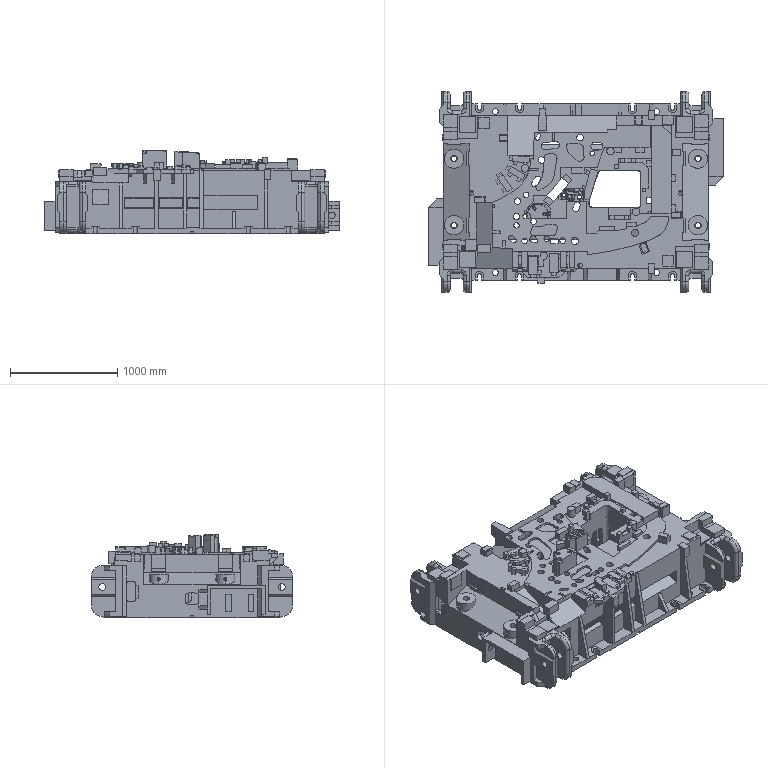Part | NX | features solid 2 | 1 solid | 2203 faces | box 2740 x 1870 x 775.227 mm | volume 830431815 mm3 | plane 1570 | cylinder 321 | spline 280 | torus 32 | commonest cylinder face diameters 80 x84 60 x81 40 x26 50 x20 30 x18 200 x16